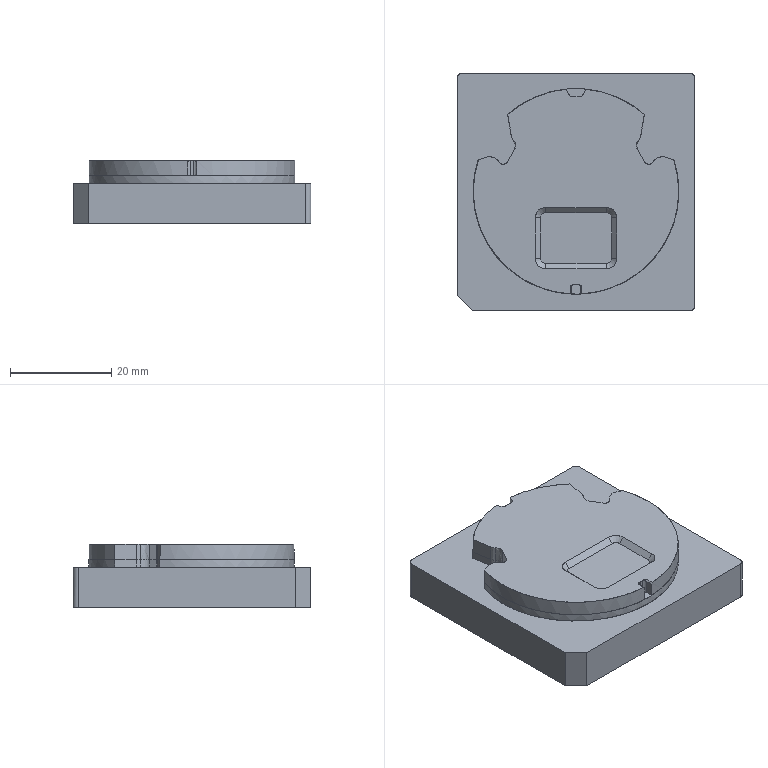NC program | PowerMill | posted with a generic post | part box 47 x 47 x 12.511 mm
Lines 10317 to 11237 of 154620:
N10414 M6
N10415 S22000 M03
N10416 G00 G90 X0.0 Y0.0
N10417 G43 Z9.8015 H27
N10418
N10419 G05 P10000 R4
N10420 X1.2281 Y-20.6433
N10421 Z0.8132
N10422 G01 Z-0.3868 F1200.0
N10423 Y-20.6295 F2000.0
N10424 G03 X1.1043 Y-20.5058 I-0.1238 J0.0
N10425 G01 X1.0305
N10426 X0.965 Y-20.4824
N10427 X0.7677 Y-20.2645
N10428 X0.7483 Y-20.0233
N10429 Y-19.7037
N10430 X0.2787 Y-19.719
N10431 G02 X0.0855 Y-19.9255 I-0.1999 J-0.0066
N10432 G01 X-0.0681 Y-19.9306
N10433 G02 X-0.2748 Y-19.7272 I-0.0068 J0.1998
N10434 G01 X-0.268 Y-19.3394
N10435 G02 X-0.0632 Y-19.143 I0.2 J-0.0035
N10436 G01 X0.0712 Y-19.1463
N10437 G02 X0.2663 Y-19.3397 I-0.0048 J-0.1999
N10438 G01 X0.2787 Y-19.719
N10439 X0.7483 Y-19.7037
N10440 Y-19.0583
N10441 X0.7247 Y-18.8611
N10442 X0.7113 Y-18.8327
N10443 X0.6506 Y-18.7685
N10444 X0.4825 Y-18.6871
N10445 X0.3623 Y-18.6688
N10446 X-0.2412 Y-18.6551
N10447 X-0.4825 Y-18.6871
N10448 X-0.6024 Y-18.7385
N10449 X-0.7073 Y-18.8225
N10450 X-0.7246 Y-18.8497
N10451 X-0.7483 Y-18.9472
N10452 Y-20.0233
N10453 X-0.7677 Y-20.2645
N10454 X-0.965 Y-20.4824
N10455 X-1.0282 Y-20.5051
N10456 X-1.0954 Y-20.5079
N10457 G00 Z3.8955
N10458 G01 X1.1671 Y-20.6433 F10000.0
N10459 G00 Z0.7655
N10460 G01 Z-0.4345 F1200.0
N10461 Y-20.6295 F2000.0
N10462 G03 X1.0433 Y-20.5058 I-0.1238 J0.0
N10463 G01 X0.9718
N10464 X0.7186 Y-20.2645
N10465 X0.71 Y-19.7014
N10466 X0.2398 Y-19.7231
N10467 G02 X0.0446 Y-19.9322 I-0.1998 J-0.0092
N10468 G01 X-0.0208 Y-19.9337
N10469 G02 X-0.2253 Y-19.7303 I-0.0045 J0.2
N10470 G01 X-0.2188 Y-19.349
N10471 G02 X-0.0165 Y-19.1525 I0.2 J-0.0035
N10472 G01 X0.0249 Y-19.1529
N10473 G02 X0.2223 Y-19.3437 I-0.0024 J-0.2
N10474 G01 X0.2398 Y-19.7231
N10475 X0.71 Y-19.7014
N10476 X0.6981 Y-18.9288
N10477 X0.6777 Y-18.8566
N10478 X0.6667 Y-18.8366
N10479 X0.6155 Y-18.7798
N10480 X0.5976 Y-18.7672
N10481 X0.3645 Y-18.6698
N10482 X-0.3522
N10483 X-0.3705 Y-18.6722
N10484 X-0.593 Y-18.7613
N10485 X-0.6108 Y-18.7734
N10486 X-0.6646 Y-18.8304
N10487 X-0.676 Y-18.85
N10488 X-0.7002 Y-18.9284
N10489 Y-20.0233
N10490 X-0.7186 Y-20.2645
N10491 X-0.965 Y-20.5026
N10492 X-1.0221 Y-20.5047
N10493 G00 Z3.8477
N10494 G01 X1.1265 Y-20.6433 F10000.0
N10495 G00 Z0.7177
N10496 G01 Z-0.4823 F1200.0
N10497 Y-20.6295 F2000.0
N10498 G03 X1.0028 Y-20.5058 I-0.1237 J0.0
N10499 G01 X0.9142
N10500 X0.7237 Y-20.3708
N10501 X0.6695 Y-20.2645
N10502 X0.6498 Y-18.929
N10503 X0.608 Y-18.829
N10504 X0.5929 Y-18.8091
N10505 X0.4784 Y-18.7183
N10506 X0.3908 Y-18.6807
N10507 X0.3737 Y-18.6736
N10508 X0.3578 Y-18.671
N10509 X-0.3578
N10510 X-0.3775 Y-18.675
N10511 X-0.4776 Y-18.7178
N10512 X-0.5929 Y-18.8093
N10513 X-0.6076 Y-18.8284
N10514 X-0.6474 Y-18.9192
N10515 X-0.6516 Y-18.9386
N10516 X-0.6597 Y-19.537
N10517 X-0.1929 Y-19.5485
N10518 X-0.1876 Y-19.3345
N10519 G02 X-0.0049 Y-19.1614 I0.1775 J-0.0044
N10520 G01 X0.0177 Y-19.162
N10521 G02 X0.19 Y-19.3356 I-0.0053 J-0.1776
N10522 G01 X0.1994 Y-19.7629
N10523 G02 X0.011 Y-19.9595 I-0.1924 J-0.0042
N10524 G01 X-0.0019 Y-19.9598
N10525 G02 X-0.1982 Y-19.7626 I-0.0039 J0.1924
N10526 G01 X-0.1929 Y-19.5485
N10527 X-0.6597 Y-19.537
N10528 X-0.6695 Y-20.2645
N10529 X-0.7237 Y-20.3708
N10530 X-0.9131 Y-20.5058
N10531 X-0.9957 Y-20.5074
N10532 G00 Z3.8
N10533 G01 X1.0982 Y-20.6433 F10000.0
N10534 G00 Z0.67
N10535 G01 Z-0.53 F1200.0
N10536 Y-20.6295 F2000.0
N10537 G03 X0.9745 Y-20.5058 I-0.1237 J0.0
N10538 G01 X0.8566
N10539 X0.7237 Y-20.4267
N10540 X0.6204 Y-20.2645
N10541 X0.6017 Y-18.9291
N10542 X0.5865 Y-18.8606
N10543 X0.575 Y-18.8382
N10544 X0.4825 Y-18.7345
N10545 X0.3836 Y-18.6786
N10546 X0.3449 Y-18.6699
N10547 X0.3053 Y-18.671
N10548 X-0.3016
N10549 X-0.4153 Y-18.6923
N10550 X-0.4203 Y-18.6936
N10551 X-0.4251 Y-18.6953
N10552 X-0.4333 Y-18.6988
N10553 X-0.4413 Y-18.7032
N10554 X-0.4484 Y-18.7091
N10555 X-0.5734 Y-18.8368
N10556 X-0.5864 Y-18.8608
N10557 X-0.6017 Y-18.9292
N10558 X-0.6106 Y-19.5638
N10559 X-0.1407 Y-19.5743
N10560 X-0.1344 Y-19.2919
N10561 G02 X-0.0168 Y-19.1768 I0.1176 J-0.0026
N10562 G01 X0.0167
N10563 G02 X0.1344 Y-19.2918 I0.0 J-0.1177
N10564 G01 X0.1471 Y-19.8566
N10565 G02 X0.0153 Y-19.9916 I-0.132 J-0.0029
N10566 G01 X-0.0147
N10567 G02 X-0.147 Y-19.8567 I-0.0003 J0.132
N10568 G01 X-0.1407 Y-19.5743
N10569 X-0.6106 Y-19.5638
N10570 X-0.6204 Y-20.2645
N10571 X-0.7237 Y-20.4267
N10572 X-0.856 Y-20.5058
N10573 X-0.9713 Y-20.5077
N10574 G00 Z3.7522
N10575 G01 X1.0779 Y-20.6433 F10000.0
N10576 G00 Z0.6222
N10577 G01 Z-0.5778 F1200.0
N10578 Y-20.6295 F2000.0
N10579 G03 X0.9542 Y-20.5058 I-0.1237 J0.0
N10580 G01 X0.7991
N10581 X0.7237 Y-20.4632
N10582 X0.5756 Y-20.2645
N10583 X0.569 Y-19.6113
N10584 X0.1082 Y-19.616
N10585 X0.1115 Y-19.9421
N10586 X0.0863 Y-20.0041
N10587 X0.0245 Y-20.0297
N10588 X-0.0286 Y-20.0296
N10589 X-0.0903 Y-20.0037
N10590 X-0.1152 Y-19.9416
N10591 X-0.106 Y-19.2895
N10592 X-0.0821 Y-19.2336
N10593 X-0.0258 Y-19.2105
N10594 X0.0247
N10595 X0.0811 Y-19.2337
N10596 X0.1049 Y-19.2899
N10597 X0.1082 Y-19.616
N10598 X0.569 Y-19.6113
N10599 X0.5634 Y-19.0583
N10600 X0.5403 Y-18.8298
N10601 X0.5318 Y-18.8065
N10602 X0.4891 Y-18.7442
N10603 X0.4723 Y-18.7288
N10604 X0.3833 Y-18.679
N10605 X0.36 Y-18.6727
N10606 X0.2748 Y-18.6709
N10607 X-0.2997
N10608 X-0.4157 Y-18.6925
N10609 X-0.4207 Y-18.6937
N10610 X-0.4256 Y-18.6955
N10611 X-0.4333 Y-18.6988
N10612 X-0.4414 Y-18.7032
N10613 X-0.4484 Y-18.7091
N10614 X-0.5083 Y-18.7703
N10615 X-0.516 Y-18.7893
N10616 X-0.5636 Y-19.0583
N10617 X-0.5805 Y-20.2645
N10618 X-0.7237 Y-20.4632
N10619 X-0.8056 Y-20.5058
N10620 X-0.9482 Y-20.5178
N10621 G00 Z3.7044
N10622 G01 X1.1022 Y-20.6529 F10000.0
N10623 G00 Z0.5744
N10624 G01 Z-0.6256 F1200.0
N10625 X1.1016 Y-20.6392 F2000.0
N10626 G03 X0.9718 Y-20.5217 I-0.1236 J-0.0061
N10627 G01 X0.965 Y-20.522
N10628 X0.796 Y-20.5058
N10629 X0.7237 Y-20.4645
N10630 X0.5719 Y-20.2645
N10631 X0.5572 Y-19.6344
N10632 X0.0955 Y-19.6438
N10633 X0.1026 Y-19.9967
N10634 X0.0828 Y-20.0467
N10635 X0.0333 Y-20.0675
N10636 X-0.0224 Y-20.0676
N10637 X-0.0718 Y-20.047
N10638 X-0.0919 Y-19.9972
N10639 X-0.082 Y-19.2913
N10640 X-0.0579 Y-19.2347
N10641 X-0.0009 Y-19.2116
N10642 X0.0078
N10643 X0.0642 Y-19.2348
N10644 X0.0883 Y-19.2908
N10645 X0.0955 Y-19.6438
N10646 X0.5572 Y-19.6344
N10647 X0.5386 Y-18.8317
N10648 X0.53 Y-18.8049
N10649 X0.4892 Y-18.7445
N10650 X0.472 Y-18.7287
N10651 X0.383 Y-18.6795
N10652 X0.3599 Y-18.6733
N10653 X0.2452 Y-18.6709
N10654 X-0.2978
N10655 X-0.4161 Y-18.6926
N10656 X-0.4212 Y-18.6938
N10657 X-0.4261 Y-18.6956
N10658 X-0.4347 Y-18.6993
N10659 X-0.4474 Y-18.7103
N10660 X-0.509 Y-18.7849
N10661 X-0.5155 Y-18.7951
N10662 X-0.5191 Y-18.8066
N10663 X-0.5369 Y-18.9075
N10664 X-0.5531 Y-20.0233
N10665 X-0.577 Y-20.2645
N10666 X-0.7237 Y-20.4645
N10667 X-0.8011 Y-20.5058
N10668 X-0.965 Y-20.522
N10669 X-0.9701 Y-20.5216
N10670 G00 Z3.6567
N10671 G01 X1.0967 Y-20.6549 F10000.0
N10672 G00 Z0.5267
N10673 G01 Z-0.6733 F1200.0
N10674 X1.0959 Y-20.6411 F2000.0
N10675 G03 X0.9652 Y-20.5248 I-0.1236 J-0.0072
N10676 G01 X0.965
N10677 X0.7941 Y-20.5058
N10678 X0.7237 Y-20.4657
N10679 X0.5682 Y-20.2645
N10680 X0.5625 Y-19.995
N10681 X0.1016 Y-20.0047
N10682 X0.081 Y-20.0544
N10683 X0.0305 Y-20.0729
N10684 X-0.0223 Y-20.0696
N10685 X-0.0619 Y-20.0511
N10686 X-0.0782 Y-20.0104
N10687 X-0.0815 Y-19.2928
N10688 X-0.0579 Y-19.2354
N10689 X-0.0005 Y-19.2118
N10690 X0.0064
N10691 X0.0626 Y-19.235
N10692 X0.0866 Y-19.2908
N10693 X0.1016 Y-20.0047
N10694 X0.5625 Y-19.995
N10695 X0.5378 Y-18.8316
N10696 X0.5294 Y-18.805
N10697 X0.4893 Y-18.7448
N10698 X0.4717 Y-18.7286
N10699 X0.3828 Y-18.68
N10700 X0.3599 Y-18.6739
N10701 X0.2165 Y-18.6708
N10702 X-0.2951
N10703 X-0.4177 Y-18.6935
N10704 X-0.4339 Y-18.6995
N10705 X-0.4471 Y-18.7107
N10706 X-0.5091 Y-18.7852
N10707 X-0.5156 Y-18.7954
N10708 X-0.5192 Y-18.807
N10709 X-0.5369 Y-18.9068
N10710 X-0.5527 Y-20.0233
N10711 X-0.5736 Y-20.2645
N10712 X-0.7237 Y-20.4657
N10713 X-0.7965 Y-20.5058
N10714 X-0.9643 Y-20.5247
N10715 G00 Z3.6089
N10716 G01 X1.0684 Y-20.6787 F10000.0
N10717 G00 Z0.4789
N10718 G01 Z-0.7211 F1200.0
N10719 X1.0701 Y-20.665 F2000.0
N10720 G03 X0.9625 Y-20.5269 I-0.1228 J0.0153
N10721 G01 X0.7923 Y-20.5058
N10722 X0.7237 Y-20.467
N10723 X0.5675 Y-20.2645
N10724 X0.5618 Y-19.9943
N10725 X0.1015 Y-20.0044
N10726 X0.081 Y-20.0541
N10727 X0.0307 Y-20.0727
N10728 X-0.0228 Y-20.0696
N10729 X-0.0626 Y-20.051
N10730 X-0.0789 Y-20.0103
N10731 X-0.0815 Y-19.2901
N10732 X-0.0581 Y-19.2331
N10733 X-0.0013 Y-19.2092
N10734 X0.0048
N10735 X0.0615 Y-19.2321
N10736 X0.0858 Y-19.288
N10737 X0.1015 Y-20.0044
N10738 X0.5618 Y-19.9943
N10739 X0.537 Y-18.8314
N10740 X0.5288 Y-18.8051
N10741 X0.4874 Y-18.742
N10742 X0.4717 Y-18.7286
N10743 X0.3852 Y-18.6813
N10744 X0.3769 Y-18.6778
N10745 X0.3681 Y-18.6759
N10746 X0.018 Y-18.6694
N10747 X-0.332 Y-18.6776
N10748 X-0.4177 Y-18.6934
N10749 X-0.4312 Y-18.6997
N10750 X-0.4399 Y-18.705
N10751 X-0.4473 Y-18.7121
N10752 X-0.5091 Y-18.7858
N10753 X-0.5157 Y-18.7961
N10754 X-0.5194 Y-18.8078
N10755 X-0.5369 Y-18.9068
N10756 X-0.5528 Y-20.0233
N10757 X-0.5688 Y-20.2084
N10758 X-0.5701 Y-20.2645
N10759 X-0.7237 Y-20.467
N10760 X-0.792 Y-20.5058
N10761 X-0.9618 Y-20.5269
N10762 G00 Z3.5611
N10763 G01 X1.0685 Y-20.6792 F10000.0
N10764 G00 Z0.4311
N10765 G01 Z-0.7689 F1200.0
N10766 X1.0702 Y-20.6655 F2000.0
N10767 G03 X0.9628 Y-20.5274 I-0.1228 J0.0153
N10768 G01 X0.7905 Y-20.5058
N10769 X0.7237 Y-20.4683
N10770 X0.567 Y-20.2645
N10771 X0.5362 Y-18.8313
N10772 X0.5282 Y-18.8052
N10773 X0.4903 Y-18.7466
N10774 X0.4859 Y-18.7408
N10775 X0.4806 Y-18.7358
N10776 X0.4717 Y-18.7285
N10777 X0.3864 Y-18.6819
N10778 X0.3781 Y-18.6783
N10779 X0.3692 Y-18.6764
N10780 X0.017 Y-18.6695
N10781 X-0.3353 Y-18.6781
N10782 X-0.4178 Y-18.6934
N10783 X-0.427 Y-18.6973
N10784 X-0.4367 Y-18.7027
N10785 X-0.4448 Y-18.7103
N10786 X-0.5093 Y-18.7869
N10787 X-0.516 Y-18.7973
N10788 X-0.5197 Y-18.809
N10789 X-0.5336 Y-18.8742
N10790 X-0.5375 Y-18.9408
N10791 X-0.5475 Y-19.6447
N10792 X-0.0848 Y-19.6485
N10793 X-0.0818 Y-19.2893
N10794 X-0.0581 Y-19.2328
N10795 X-0.0015 Y-19.2092
N10796 X0.004
N10797 X0.0608 Y-19.2322
N10798 X0.0851 Y-19.2884
N10799 X0.0992 Y-20.0052
N10800 X0.0797 Y-20.0537
N10801 X0.0314 Y-20.0734
N10802 X-0.0241 Y-20.0728
N10803 X-0.0694 Y-20.0534
N10804 X-0.0878 Y-20.0077
N10805 X-0.0848 Y-19.6485
N10806 X-0.5475 Y-19.6447
N10807 X-0.5528 Y-20.0233
N10808 X-0.5638 Y-20.1437
N10809 X-0.567 Y-20.2645
N10810 X-0.7237 Y-20.4683
N10811 X-0.7905 Y-20.5058
N10812 X-0.9589 Y-20.5269
N10813 G00 Z3.5134
N10814 G01 X1.0673 Y-20.6796 F10000.0
N10815 G00 Z0.3834
N10816 G01 Z-0.8166 F1200.0
N10817 X1.069 Y-20.6659 F2000.0
N10818 G03 X0.9618 Y-20.5276 I-0.1228 J0.0155
N10819 G01 X0.7889 Y-20.5058
N10820 X0.7237 Y-20.4696
N10821 X0.5665 Y-20.2645
N10822 X0.5354 Y-18.8311
N10823 X0.5276 Y-18.8053
N10824 X0.4897 Y-18.7459
N10825 X0.4849 Y-18.7395
N10826 X0.479 Y-18.7341
N10827 X0.4718 Y-18.7285
N10828 X0.3883 Y-18.6829
N10829 X0.38 Y-18.6793
N10830 X0.3713 Y-18.6774
N10831 X0.0159 Y-18.6694
N10832 X-0.3393 Y-18.6788
N10833 X-0.4178 Y-18.6933
N10834 X-0.4237 Y-18.6956
N10835 X-0.434 Y-18.7011
N10836 X-0.4427 Y-18.7091
N10837 X-0.5095 Y-18.7881
N10838 X-0.5162 Y-18.7985
N10839 X-0.5199 Y-18.8102
N10840 X-0.5375 Y-18.9161
N10841 X-0.5387 Y-19.0234
N10842 X-0.5475 Y-19.6442
N10843 X-0.0851 Y-19.6484
N10844 X-0.0819 Y-19.2892
N10845 X-0.0581 Y-19.2327
N10846 X-0.0015 Y-19.2092
N10847 X0.0034
N10848 X0.0601 Y-19.2321
N10849 X0.0844 Y-19.2882
N10850 X0.0992 Y-20.005
N10851 X0.0798 Y-20.0536
N10852 X0.0315 Y-20.0734
N10853 X-0.0247 Y-20.0727
N10854 X-0.07 Y-20.0533
N10855 X-0.0884 Y-20.0076
N10856 X-0.0851 Y-19.6484
N10857 X-0.5475 Y-19.6442
N10858 X-0.5529 Y-20.0233
N10859 X-0.5635 Y-20.1437
N10860 X-0.5665 Y-20.2645
N10861 X-0.7237 Y-20.4696
N10862 X-0.7891 Y-20.5058
N10863 X-0.9579 Y-20.5271
N10864 G00 Z3.4656
N10865 G01 X1.0679 Y-20.6802 F10000.0
N10866 G00 Z0.3356
N10867 G01 Z-0.8644 F1200.0
N10868 X1.0696 Y-20.6666 F2000.0
N10869 G03 X0.9625 Y-20.5281 I-0.1227 J0.0157
N10870 G01 X0.7874 Y-20.5058
N10871 X0.7237 Y-20.4709
N10872 X0.5659 Y-20.2645
N10873 X0.5653 Y-20.208
N10874 X0.5355 Y-18.8311
N10875 X0.5332 Y-18.8171
N10876 X0.5287 Y-18.8081
N10877 X0.4883 Y-18.7439
N10878 X0.4825 Y-18.7364
N10879 X0.4718 Y-18.7284
N10880 X0.3895 Y-18.6835
N10881 X0.3812 Y-18.6799
N10882 X0.3725 Y-18.678
N10883 X0.0149 Y-18.6694
N10884 X-0.3426 Y-18.6794
N10885 X-0.414 Y-18.6926
N10886 X-0.4286 Y-18.6979
N10887 X-0.4407 Y-18.7077
N10888 X-0.4633 Y-18.7333
N10889 X-0.5096 Y-18.788
N10890 X-0.5162 Y-18.7984
N10891 X-0.52 Y-18.8102
N10892 X-0.5341 Y-18.8901
N10893 X-0.5364 Y-19.0845
N10894 X-0.5394 Y-19.2788
N10895 X-0.0824 Y-19.2885
N10896 X-0.0582 Y-19.2324
N10897 X-0.0017 Y-19.2092
N10898 X0.0016
N10899 X0.0585 Y-19.2322
N10900 X0.0829 Y-19.2885
N10901 X0.0979 Y-20.0051
N10902 X0.0781 Y-20.0552
N10903 X0.0285 Y-20.076
N10904 X-0.0283 Y-20.0759
N10905 X-0.0778 Y-20.0551
N10906 X-0.0976 Y-20.0051
N10907 X-0.0824 Y-19.2885
N10908 X-0.5394 Y-19.2788
N10909 X-0.5503 Y-19.7717
N10910 X-0.5659 Y-20.2645
N10911 X-0.7237 Y-20.4709
N10912 X-0.7877 Y-20.5058
N10913 X-0.9581 Y-20.5276
N10914 G00 Z3.4179
N10915 G01 X1.0673 Y-20.6807 F10000.0
N10916 G00 Z0.2878
N10917 G01 Z-0.9122 F1200.0
N10918 X1.0691 Y-20.667 F2000.0
N10919 G03 X0.9621 Y-20.5285 I-0.1228 J0.0158
N10920 G01 X0.7859 Y-20.5058
N10921 X0.7237 Y-20.4722
N10922 X0.5654 Y-20.2645
N10923 X0.5641 Y-20.1525
N10924 X0.5356 Y-18.8362
N10925 X0.5348 Y-18.8285
N10926 X0.5328 Y-18.8211
N10927 X0.5281 Y-18.8082
N10928 X0.4885 Y-18.7443
N10929 X0.4804 Y-18.7344
N10930 X0.4718 Y-18.7284
N10931 X0.3826 Y-18.6797
N10932 X-0.0172 Y-18.6686
N10933 X-0.4165 Y-18.693
N10934 X-0.4428 Y-18.7097
N10935 X-0.4633 Y-18.7333
N10936 X-0.5096 Y-18.788
N10937 X-0.5163 Y-18.7984
N10938 X-0.52 Y-18.8102
N10939 X-0.5338 Y-18.8879
N10940 X-0.5365 Y-19.0826
N10941 X-0.5398 Y-19.2772
N10942 X-0.082 Y-19.2875
N10943 X-0.0581 Y-19.2318
N10944 X-0.0022 Y-19.2083
N10945 X0.0002 Y-19.2082
N10946 X0.0576 Y-19.2309
N10947 X0.0824 Y-19.2874
N10948 X0.0984 Y-20.0058
N10949 X0.0786 Y-20.0559
N10950 X0.029 Y-20.0767
N10951 X-0.0288
N10952 X-0.0784 Y-20.0558
N10953 X-0.0981 Y-20.0057
N10954 X-0.082 Y-19.2875
N10955 X-0.5398 Y-19.2772
N10956 X-0.5508 Y-19.7709
N10957 X-0.5654 Y-20.2645
N10958 X-0.7237 Y-20.4722
N10959 X-0.7862 Y-20.5058
N10960 X-0.9577 Y-20.5279
N10961 G00 Z3.3701
N10962 G01 X1.0667 Y-20.6811 F10000.0
N10963 G00 Z0.2401
N10964 G01 Z-0.9599 F1200.0
N10965 X1.0685 Y-20.6675 F2000.0
N10966 G03 X0.9617 Y-20.5288 I-0.1227 J0.016
N10967 G01 X0.7844 Y-20.5058
N10968 X0.7237 Y-20.4734
N10969 X0.5648 Y-20.2645
N10970 X0.563 Y-20.098
N10971 X0.5609 Y-20.002
N10972 X0.0968 Y-20.0107
N10973 X0.0771 Y-20.0583
N10974 X0.0289 Y-20.0764
N10975 X-0.0232 Y-20.0736
N10976 X-0.0616 Y-20.0559
N10977 X-0.0773 Y-20.0166
N10978 X-0.0793 Y-19.291
N10979 X-0.0567 Y-19.2348
N10980 X-0.0012 Y-19.2101
N10981 X-0.0002
N10982 X0.0581 Y-19.2322
N10983 X0.0832 Y-19.2893
N10984 X0.0968 Y-20.0107
N10985 X0.5609 Y-20.002
N10986 X0.5357 Y-18.8364
N10987 X0.5343 Y-18.8271
N10988 X0.5133 Y-18.7796
N10989 X0.4827 Y-18.7377
N10990 X0.4766 Y-18.7318
N10991 X0.4696 Y-18.7271
N10992 X0.3845 Y-18.6807
N10993 X0.191 Y-18.6687
N10994 X-0.0029 Y-18.6705
N10995 X-0.3501 Y-18.6807
N10996 X-0.415 Y-18.6926
N10997 X-0.4422 Y-18.7094
N10998 X-0.4633 Y-18.7332
N10999 X-0.5096 Y-18.788
N11000 X-0.5163 Y-18.7984
N11001 X-0.52 Y-18.8101
N11002 X-0.5331 Y-18.8835
N11003 X-0.543 Y-19.3138
N11004 X-0.553 Y-20.0233
N11005 X-0.5627 Y-20.1437
N11006 X-0.5648 Y-20.2645
N11007 X-0.7237 Y-20.4734
N11008 X-0.7848 Y-20.5058
N11009 X-0.9573 Y-20.5283
N11010 G00 Z3.3223
N11011 G01 X1.0661 Y-20.6816 F10000.0
N11012 G00 Z0.1923
N11013 G01 Z-1.0077 F1200.0
N11014 X1.0679 Y-20.668 F2000.0
N11015 G03 X0.9613 Y-20.5292 I-0.1227 J0.0161
N11016 G01 X0.7829 Y-20.5058
N11017 X0.7237 Y-20.4747
N11018 X0.5643 Y-20.2645
N11019 X0.5619 Y-20.0445
N11020 X0.561 Y-20.0022
N11021 X0.0967 Y-20.0114
N11022 X0.0771 Y-20.059
N11023 X0.0289 Y-20.0771
N11024 X-0.0237 Y-20.0743
N11025 X-0.0622 Y-20.0566
N11026 X-0.0779 Y-20.0173
N11027 X-0.0791 Y-19.2916
N11028 X-0.0564 Y-19.2352
N11029 X-0.0009 Y-19.2107
N11030 X-0.0008
N11031 X0.0573 Y-19.2329
N11032 X0.0825 Y-19.2898
N11033 X0.0967 Y-20.0114
N11034 X0.561 Y-20.0022
N11035 X0.5359 Y-18.8422
N11036 X0.5334 Y-18.8262
N11037 X0.5312 Y-18.8174
N11038 X0.5273 Y-18.8091
N11039 X0.4888 Y-18.7451
N11040 X0.4805 Y-18.736
N11041 X0.4748 Y-18.7307
N11042 X0.4683 Y-18.7264
N11043 X0.3864 Y-18.6816
N11044 X0.2011 Y-18.6688
N11045 X0.0154 Y-18.6705
N11046 X-0.3542 Y-18.6814
N11047 X-0.4135 Y-18.6923
N11048 X-0.4415 Y-18.709
N11049 X-0.4634 Y-18.7332
N11050 X-0.5097 Y-18.7879
N11051 X-0.5163 Y-18.7983
N11052 X-0.5201 Y-18.8101
N11053 X-0.5327 Y-18.8813
N11054 X-0.5437 Y-19.3628
N11055 X-0.5531 Y-20.0233
N11056 X-0.5625 Y-20.1437
N11057 X-0.5643 Y-20.2645
N11058 X-0.7237 Y-20.4747
N11059 X-0.7834 Y-20.5058
N11060 X-0.9569 Y-20.5286
N11061 G00 Z3.2746
N11062 G01 X1.0656 Y-20.6821 F10000.0
N11063 G00 Z0.1446
N11064 G01 Z-1.0554 F1200.0
N11065 X1.0674 Y-20.6684 F2000.0
N11066 G03 X0.9609 Y-20.5295 I-0.1227 J0.0162
N11067 G01 X0.7815 Y-20.5058
N11068 X0.7237 Y-20.476
N11069 X0.5637 Y-20.2645
N11070 X0.5536 Y-19.5407
N11071 X0.5313 Y-18.8171
N11072 X0.4889 Y-18.7455
N11073 X0.4779 Y-18.7341
N11074 X0.4726 Y-18.7293
N11075 X0.4666 Y-18.7254
N11076 X0.3952 Y-18.6864
N11077 X0.387 Y-18.6829
N11078 X0.3784 Y-18.681
N11079 X0.2053 Y-18.669
N11080 X0.0317 Y-18.6704
N11081 X-0.3576 Y-18.6819
N11082 X-0.4039 Y-18.6891
N11083 X-0.4448 Y-18.712
N11084 X-0.4634 Y-18.7332
N11085 X-0.5097 Y-18.7879
N11086 X-0.5164 Y-18.7983
N11087 X-0.5201 Y-18.8101
N11088 X-0.532 Y-18.8771
N11089 X-0.5448 Y-19.4349
N11090 X-0.5478 Y-19.6493
N11091 X-0.0816 Y-19.6527
N11092 X-0.0789 Y-19.2913
N11093 X-0.0559 Y-19.2354
N11094 X-0.0005 Y-19.2112
N11095 X0.0019 Y-19.2111
N11096 X0.06 Y-19.2333
N11097 X0.0851 Y-19.2903
N11098 X0.0995 Y-20.0099
N11099 X0.0797 Y-20.0587
N11100 X0.0307 Y-20.0781
N11101 X-0.024 Y-20.0766
N11102 X-0.0669 Y-20.0577
N11103 X-0.0843 Y-20.0141
N11104 X-0.0816 Y-19.6527
N11105 X-0.5478 Y-19.6493
N11106 X-0.5531 Y-20.0233
N11107 X-0.5623 Y-20.1437
N11108 X-0.5638 Y-20.2645
N11109 X-0.7237 Y-20.476
N11110 X-0.7819 Y-20.5058
N11111 X-0.9566 Y-20.5289
N11112 G00 Z3.2268
N11113 G01 X1.0644 Y-20.6824 F10000.0
N11114 G00 Z0.0968
N11115 G01 Z-1.1032 F1200.0
N11116 X1.0662 Y-20.6688 F2000.0
N11117 G03 X0.9599 Y-20.5298 I-0.1226 J0.0164
N11118 G01 X0.78 Y-20.5058
N11119 X0.7237 Y-20.4773
N11120 X0.5632 Y-20.2645
N11121 X0.5534 Y-19.5407
N11122 X0.5305 Y-18.8171
N11123 X0.489 Y-18.7459
N11124 X0.4759 Y-18.7327
N11125 X0.4708 Y-18.7282
N11126 X0.4651 Y-18.7245
N11127 X0.3966 Y-18.6871
N11128 X0.3885 Y-18.6836
N11129 X0.3799 Y-18.6817
N11130 X0.2153 Y-18.6692
N11131 X0.0503 Y-18.6704
N11132 X-0.3623 Y-18.6828
N11133 X-0.4027 Y-18.6902
N11134 X-0.4108 Y-18.6925
N11135 X-0.4183 Y-18.6961
N11136 X-0.4385 Y-18.7082
N11137 X-0.4445 Y-18.7124
N11138 X-0.4497 Y-18.7175
N11139 X-0.4634 Y-18.7331
N11140 X-0.5098 Y-18.7879
N11141 X-0.5164 Y-18.7983
N11142 X-0.5202 Y-18.81
N11143 X-0.5314 Y-18.8733
N11144 X-0.5458 Y-19.503
N11145 X-0.5516 Y-19.9117
N11146 X-0.0915 Y-19.9201
N11147 X-0.08 Y-19.2911
N11148 X-0.0567 Y-19.2357
N11149 X-0.0015 Y-19.2117
N11150 X0.0013 Y-19.2116
N11151 X0.0597 Y-19.234
N11152 X0.0847 Y-19.2912
N11153 X0.0963 Y-20.0102
N11154 X0.0771 Y-20.0583
N11155 X0.0293 Y-20.0782
N11156 X-0.0263 Y-20.0781
N11157 X-0.074 Y-20.058
N11158 X-0.0931 Y-20.01
N11159 X-0.0915 Y-19.9201
N11160 X-0.5516 Y-19.9117
N11161 X-0.5532 Y-20.0233
N11162 X-0.562 Y-20.1437
N11163 X-0.5632 Y-20.2645
N11164 X-0.7237 Y-20.4773
N11165 X-0.7805 Y-20.5058
N11166 X-0.9556 Y-20.5292
N11167 G00 Z3.179
N11168 G01 X1.0644 Y-20.683 F10000.0
N11169 G00 Z0.049
N11170 G01 Z-1.151 F1200.0
N11171 X1.0662 Y-20.6693 F2000.0
N11172 G03 X0.9601 Y-20.5302 I-0.1226 J0.0165
N11173 G01 X0.7785 Y-20.5058
N11174 X0.7237 Y-20.478
N11175 X0.5627 Y-20.2645
N11176 X0.5531 Y-19.5411
N11177 X0.5298 Y-18.818
N11178 X0.489 Y-18.7469
N11179 X0.4469 Y-18.7125
N11180 X0.3984 Y-18.688
N11181 X0.3903 Y-18.6845
N11182 X0.3817 Y-18.6826
N11183 X0.2244 Y-18.6694
N11184 X0.0666 Y-18.6703
N11185 X-0.3658 Y-18.6834
N11186 X-0.4207 Y-18.6964
N11187 X-0.4635 Y-18.7331
N11188 X-0.5098 Y-18.7879
N11189 X-0.5165 Y-18.7982
N11190 X-0.5202 Y-18.81
N11191 X-0.5314 Y-18.8733
N11192 X-0.5458 Y-19.503
N11193 X-0.5517 Y-19.9128
N11194 X-0.0918 Y-19.9215
N11195 X-0.0799 Y-19.2915
N11196 X-0.0565 Y-19.2362
N11197 X-0.0014 Y-19.2122
N11198 X0.001 Y-19.2121
N11199 X0.0593 Y-19.2344
N11200 X0.0843 Y-19.2916
N11201 X0.0967 Y-20.0117
N11202 X0.0775 Y-20.0598
N11203 X0.0297 Y-20.0798
N11204 X-0.0267 Y-20.0797
N11205 X-0.0744 Y-20.0596
N11206 X-0.0935 Y-20.0114
N11207 X-0.0918 Y-19.9215
N11208 X-0.5517 Y-19.9128
N11209 X-0.5532 Y-20.0233
N11210 X-0.5613 Y-20.1438
N11211 X-0.5627 Y-20.2645
N11212 X-0.7237 Y-20.478
N11213 X-0.7791 Y-20.5058
N11214 X-0.9564 Y-20.5297
N11215 G00 Z3.1313
N11216 G01 X1.0638 Y-20.6834 F10000.0
N11217 G00 Z0.0013
N11218 G01 Z-1.1987 F1200.0
N11219 X1.0656 Y-20.6698 F2000.0
N11220 G03 X0.9596 Y-20.5305 I-0.1226 J0.0166
N11221 G01 X0.777 Y-20.5058
N11222 X0.7237 Y-20.4787
N11223 X0.5621 Y-20.2645
N11224 X0.5529 Y-19.5411
N11225 X0.5291 Y-18.8179
N11226 X0.489 Y-18.7478
N11227 X0.4477 Y-18.7137
N11228 X0.4003 Y-18.689
N11229 X0.3922 Y-18.6855
N11230 X0.3836 Y-18.6836
N11231 X0.2341 Y-18.6697
N11232 X0.0839 Y-18.6703
N11233 X-0.3703 Y-18.6841
N11234 X-0.3982 Y-18.6893
N11235 X-0.4058 Y-18.6914
N11236 X-0.413 Y-18.6947
N11237 X-0.4415 Y-18.7097
N11238 X-0.4635 Y-18.7331
N11239 X-0.5099 Y-18.7878
N11240 X-0.5165 Y-18.7982
N11241 X-0.5202 Y-18.81
N11242 X-0.5315 Y-18.8733
N11243 X-0.5459 Y-19.503
N11244 X-0.5479 Y-19.6475
N11245 X-0.0848 Y-19.6538
N11246 X-0.0798 Y-19.2933
N11247 X-0.0569 Y-19.238
N11248 X-0.0021 Y-19.2136
N11249 X-0.0001 Y-19.2135
N11250 X0.0586 Y-19.2355
N11251 X0.084 Y-19.2929
N11252 X0.0971 Y-20.0123
N11253 X0.0776 Y-20.0608
N11254 X0.0292 Y-20.0805
N11255 X-0.0262 Y-20.0797
N11256 X-0.0715 Y-20.0601
N11257 X-0.0897 Y-20.0143
N11258 X-0.0848 Y-19.6538
N11259 X-0.5479 Y-19.6475
N11260 X-0.5533 Y-20.0233
N11261 X-0.561 Y-20.1438
N11262 X-0.5621 Y-20.2645
N11263 X-0.7237 Y-20.4787
N11264 X-0.7776 Y-20.5058
N11265 X-0.956 Y-20.53
N11266 G00 Z3.0835
N11267 G01 X1.0637 Y-20.6834 F10000.0
N11268 G00 Z-0.0465
N11269 G01 Z-1.2465 F1200.0
N11270 X1.0655 Y-20.6697 F2000.0
N11271 G03 X0.9595 Y-20.5305 I-0.1226 J0.0166
N11272 G01 X0.777 Y-20.5057
N11273 X0.7311 Y-20.4823
N11274 X0.7275 Y-20.4807
N11275 X0.7237 Y-20.4794
N11276 X0.5616 Y-20.2645
N11277 X0.5527 Y-19.5414
N11278 X0.5286 Y-18.8187
N11279 X0.4889 Y-18.7489
N11280 X0.442 Y-18.71
N11281 X0.3866 Y-18.6847
N11282 X0.2441 Y-18.6702
N11283 X0.1009
N11284 X-0.3748 Y-18.6849
N11285 X-0.3965 Y-18.6889
N11286 X-0.4042 Y-18.691
N11287 X-0.4114 Y-18.6944
N11288 X-0.4407 Y-18.7094
N11289 X-0.4636 Y-18.733
N11290 X-0.5123 Y-18.7907
N11291 X-0.5188 Y-18.8016
N11292 X-0.5315 Y-18.8733
N11293 X-0.5459 Y-19.503
N11294 X-0.548 Y-19.6476
N11295 X-0.0849 Y-19.6543
N11296 X-0.0797 Y-19.2936
N11297 X-0.0567 Y-19.2383
N11298 X-0.0019 Y-19.214
N11299 X-0.0002 Y-19.2139
N11300 X0.0584 Y-19.236
N11301 X0.0837 Y-19.2932
N11302 X0.0976 Y-20.013
N11303 X0.0781 Y-20.0615
N11304 X0.0297 Y-20.0812
N11305 X-0.0265 Y-20.0804
N11306 X-0.0719 Y-20.0608
N11307 X-0.0901 Y-20.0149
N11308 X-0.0849 Y-19.6543
N11309 X-0.548 Y-19.6476
N11310 X-0.5533 Y-20.0233
N11311 X-0.5614 Y-20.1438
N11312 X-0.5616 Y-20.2645
N11313 X-0.7237 Y-20.4794
N11314 X-0.7263 Y-20.4799
N11315 X-0.7777 Y-20.5057
N11316 X-0.9559 Y-20.53
N11317 G00 Z3.0357
N11318 G01 X1.0506 Y-20.6912 F10000.0
N11319 G00 Z-0.0943
N11320 G01 Z-1.2943 F1200.0
N11321 X1.0535 Y-20.6777 F2000.0
N11322 G03 X0.9586 Y-20.5307 I-0.121 J0.026
N11323 G01 X0.9537 Y-20.5296
N11324 X0.7771 Y-20.5057
N11325 X0.7288 Y-20.4811
N11326 X0.7237 Y-20.4801
N11327 X0.561 Y-20.2645
N11328 X0.5529 Y-19.5677
N11329 X0.5368 Y-18.871
N11330 X0.528 Y-18.8186
N11331 X0.4874 Y-18.7478
N11332 X0.4756 Y-18.7354
N11333 X0.4708 Y-18.731
N11334 X0.4655 Y-18.7273